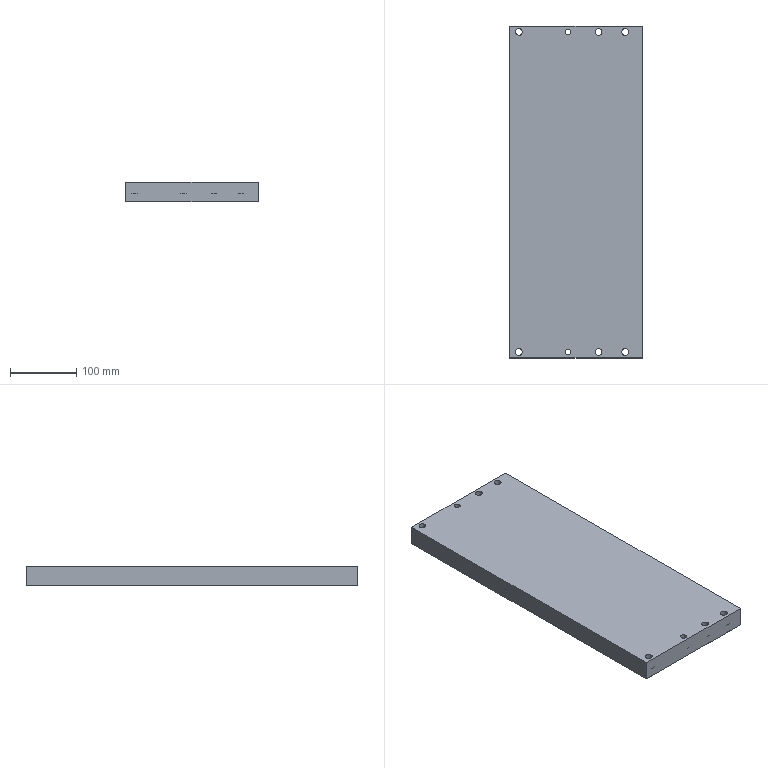CAM job | NX | 3-axis milling, drilling | part box 200 x 500 x 30 mm | stock box 200 x 500 x 30 mm
Tools:
number,name,description,diameter,corner_radius,flute_length,length,flutes
0,D18R0,Milling Tool-5 Parameters,18.0,0.0,50.0,75.0,2
14,D10R0,Milling Tool-5 Parameters,10.0,0.0,50.0,75.0,2
2,D11Z,Drilling Tool,11.0,0.0,35.0,50.0,2
12,D10.3Z,Drilling Tool,10.3,0.0,35.0,50.0,2
0,D10.5Z,Drilling Tool,10.5,0.0,35.0,50.0,2
10,D8.5Z,Drilling Tool,8.5,0.0,35.0,50.0,2
1,DJ-6,Countersink,6.0,0.0,0.0,60.0,2
2,ZXZ,Centerdrill,8.0,0.0,0.0,50.0,2
1,DJ-12,Countersink,12.0,0.0,0.0,60.0,2
0,M10,Drilling Tool,10.0,0.0,35.0,50.0,4
0,M12,Drilling Tool,12.0,0.0,35.0,50.0,4
3,D10,Milling Tool-5 Parameters,10.0,0.0,50.0,75.0,2
Operations:
program,operation,operation_type,tool,method,geometry_group,spindle_rpm,surface_speed,feed_per_tooth,feed_cut,feed_plunge,cut_length_mm,path_length_mm,cut_time_min,machine_time_min
A01,DRILLING,Operation,ZXZ,METHOD,MCS_MILL,1000.0,25.0,0.03,60.0,0.0,12.0,708.497,0.2,0.2696
A02,DRILLING_COPY,Operation,D10.5Z,METHOD,MCS_MILL,650.0,21.0,0.0462,60.0,0.0,126.0,936.497,2.1,2.181
A03,DRILLING_COPY_COPY,Operation,D18R0,METHOD,MCS_MILL,400.0,13.0,0.0375,30.0,0.0,54.0,792.497,1.8,1.874
A05,PLANAR_MILL,PlanarMilling,D10R0,METHOD,MCS_MILL,2500.0,78.0,0.08,400.0,100.0,443.101,896.248,1.108,1.2
A06,PLANAR_MILL_COPY,PlanarMilling,DJ-6,METHOD,MCS_MILL,3000.0,56.0,0.1333,800.0,100.0,231.929,1252.796,0.2899,0.4685
A06,PLANAR_MILL_COPY_COPY,PlanarMilling,DJ-6,METHOD,MCS_MILL,3000.0,56.0,0.1333,800.0,100.0,447.101,822.448,0.5589,0.6347
B01,DRILLING_COPY_1,Operation,ZXZ,METHOD,MCS_MILL,1000.0,25.0,0.03,60.0,0.0,9.0,508.88,0.15,0.2
B02,DRILLING_COPY_1_COPY,Operation,D8.5Z,METHOD,MCS_MILL,800.0,21.0,0.0375,60.0,0.0,69.0,628.88,1.15,1.206
B03,DRILLING_COPY_1_COPY_COPY,Operation,M10,METHOD,MCS_MILL,100.0,2.0,0.0075,1.5,0.0,34.5,559.88,23.0,23.052
C01,DRILLING_COPY_1_COPY_1,Operation,ZXZ,METHOD,MCS_MILL,1000.0,25.0,0.03,60.0,0.0,18.0,1029.821,0.3,0.4012
C02,DRILLING_COPY_1_COPY_COPY_1,Operation,D8.5Z,METHOD,MCS_MILL,800.0,21.0,0.0375,60.0,0.0,79.5,649.88,1.325,1.382
C03,DRILLING_COPY_1_COPY_COPY_COPY,Operation,D10.3Z,METHOD,MCS_MILL,500.0,16.0,0.0215,21.5,0.0,69.0,691.665,3.209,3.272
C04,DRILLING_COPY_1_COPY_COPY_COPY_1,Operation,M10,METHOD,MCS_MILL,100.0,2.0,0.0075,1.5,0.0,34.5,559.88,23.0,23.052
C05,DRILLING_COPY_1_COPY_COPY_COPY_1_COPY,Operation,M12,METHOD,MCS_MILL,100.0,2.0,0.0075,1.5,0.0,34.5,622.665,23.0,23.059
过桥板,DJ,Operation,DJ-12,METHOD,WORKPIECE_111111,2000.0,75.0,0.03,120.0,0.0,56.0,1234.469,0.4667,0.5845
过桥板,11ZT,Operation,D11Z,METHOD,WORKPIECE_111111,2000.0,75.0,0.03,120.0,0.0,296.0,1714.469,2.467,2.608
过桥板,PLANAR_MILL_1,PlanarMilling,D10,METHOD,WORKPIECE_111111,3500.0,109.0,0.0429,300.0,100.0,3219.657,4616.802,10.732,10.872
过桥板,PLANAR_MILL_1_COPY,PlanarMilling,D10,METHOD,WORKPIECE_111111,3500.0,109.0,0.0429,300.0,100.0,274.195,1718.941,0.914,1.058
过桥板,DJ-J,PlanarMilling,DJ-6,METHOD,WORKPIECE_111111,3000.0,56.0,0.1667,1000.0,100.0,501.169,1778.022,0.5012,0.6289
过桥板,DJ-J_COPY,PlanarMilling,DJ-6,METHOD,WORKPIECE_111111,3000.0,56.0,0.1667,1000.0,100.0,240.894,1708.18,0.2409,0.3876